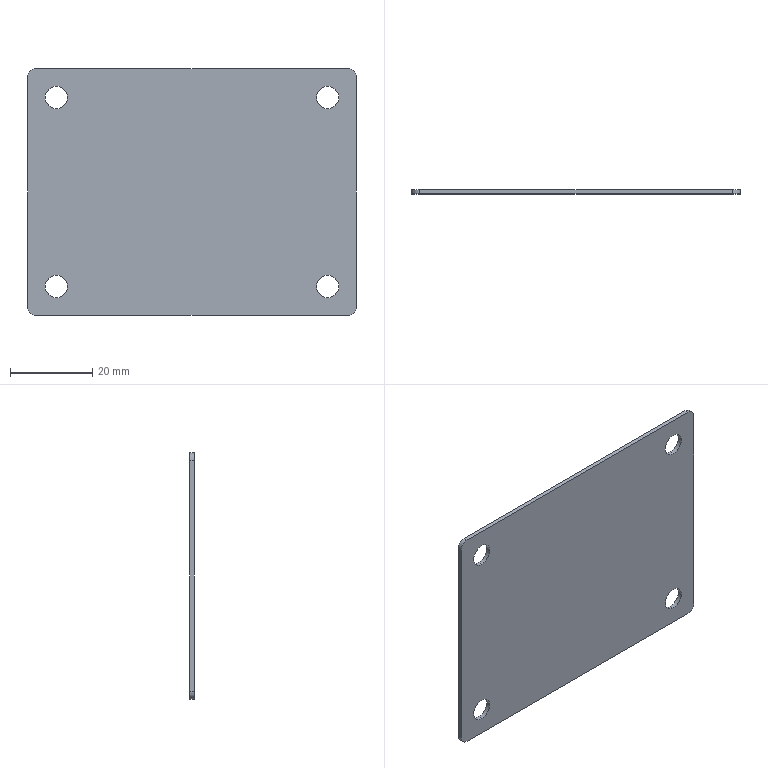Part | STEP file | 4060 profile end cover plate | 1 solid | 18 faces | box 80 x 1 x 60 mm | volume 4702 mm3 | cylinder 12 | plane 6 | commonest cylinder face diameters 5.5 x8 4 x4
STEP:
#1=CARTESIAN_POINT('',(0.,0.,0.));
#2=DIRECTION('',(0.,0.,1.));
#3=DIRECTION('',(1.,0.,0.));
#4=AXIS2_PLACEMENT_3D('',#1,#2,#3);
#5=CARTESIAN_POINT('',(33.,0.,-20.25));
#6=VERTEX_POINT('',#5);
#7=CARTESIAN_POINT('',(33.,1.,-20.25));
#8=VERTEX_POINT('',#7);
#9=CARTESIAN_POINT('',(33.,1.,-20.25));
#10=DIRECTION('',(0.,1.,0.));
#11=VECTOR('',#10,1.);
#12=LINE('',#9,#11);
#13=CARTESIAN_POINT('',(33.,1.,-23.));
#14=DIRECTION('',(0.,1.,0.));
#15=DIRECTION('',(0.,0.,1.));
#16=AXIS2_PLACEMENT_3D('',#13,#14,#15);
#17=CYLINDRICAL_SURFACE('',#16,2.75);
#18=CARTESIAN_POINT('',(6.283,0.));
#19=DIRECTION('',(0.,1.));
#20=VECTOR('',#19,1.);
#21=LINE('',#18,#20);
#22=(GEOMETRIC_REPRESENTATION_CONTEXT(2)PARAMETRIC_REPRESENTATION_CONTEXT()REPRESENTATION_CONTEXT('',''));
#23=DEFINITIONAL_REPRESENTATION('',(#21),#22);
#24=PCURVE('',#17,#23);
#25=CARTESIAN_POINT('',(33.,1.,-23.));
#26=DIRECTION('',(0.,1.,0.));
#27=DIRECTION('',(0.,0.,1.));
#28=AXIS2_PLACEMENT_3D('',#25,#26,#27);
#29=CYLINDRICAL_SURFACE('',#28,2.75);
#30=CARTESIAN_POINT('',(0.,0.));
#31=DIRECTION('',(0.,1.));
#32=VECTOR('',#31,1.);
#33=LINE('',#30,#32);
#34=(GEOMETRIC_REPRESENTATION_CONTEXT(2)PARAMETRIC_REPRESENTATION_CONTEXT()REPRESENTATION_CONTEXT('',''));
#35=DEFINITIONAL_REPRESENTATION('',(#33),#34);
#36=PCURVE('',#29,#35);
#37=SURFACE_CURVE('',#12,(#24,#36),.PCURVE_S1.);
#38=EDGE_CURVE('',#6,#8,#37,.T.);
#39=ORIENTED_EDGE('',*,*,#38,.T.);
#40=CARTESIAN_POINT('',(33.,1.,-25.75));
#41=VERTEX_POINT('',#40);
#42=CARTESIAN_POINT('',(33.,1.,-23.));
#43=DIRECTION('',(0.,1.,0.));
#44=DIRECTION('',(0.,0.,1.));
#45=AXIS2_PLACEMENT_3D('',#42,#43,#44);
#46=CIRCLE('',#45,2.75);
#47=CARTESIAN_POINT('',(0.,0.));
#48=DIRECTION('',(1.,0.));
#49=VECTOR('',#48,1.);
#50=LINE('',#47,#49);
#51=(GEOMETRIC_REPRESENTATION_CONTEXT(2)PARAMETRIC_REPRESENTATION_CONTEXT()REPRESENTATION_CONTEXT('',''));
#52=DEFINITIONAL_REPRESENTATION('',(#50),#51);
#53=PCURVE('',#17,#52);
#54=CARTESIAN_POINT('',(-38.,1.,28.));
#55=DIRECTION('',(0.,1.,0.));
#56=DIRECTION('',(0.,0.,1.));
#57=AXIS2_PLACEMENT_3D('',#54,#55,#56);
#58=PLANE('',#57);
#59=CARTESIAN_POINT('',(-51.,71.));
#60=DIRECTION('',(1.,0.));
#61=AXIS2_PLACEMENT_2D('',#59,#60);
#62=CIRCLE('',#61,2.75);
#63=(GEOMETRIC_REPRESENTATION_CONTEXT(2)PARAMETRIC_REPRESENTATION_CONTEXT()REPRESENTATION_CONTEXT('',''));
#64=DEFINITIONAL_REPRESENTATION('',(#62),#63);
#65=PCURVE('',#58,#64);
#66=SURFACE_CURVE('',#46,(#53,#65),.PCURVE_S1.);
#67=EDGE_CURVE('',#41,#8,#66,.T.);
#68=ORIENTED_EDGE('',*,*,#67,.F.);
#69=CARTESIAN_POINT('',(33.,0.,-25.75));
#70=VERTEX_POINT('',#69);
#71=CARTESIAN_POINT('',(33.,1.,-25.75));
#72=DIRECTION('',(0.,1.,0.));
#73=VECTOR('',#72,1.);
#74=LINE('',#71,#73);
#75=CARTESIAN_POINT('',(3.142,0.));
#76=DIRECTION('',(0.,1.));
#77=VECTOR('',#76,1.);
#78=LINE('',#75,#77);
#79=(GEOMETRIC_REPRESENTATION_CONTEXT(2)PARAMETRIC_REPRESENTATION_CONTEXT()REPRESENTATION_CONTEXT('',''));
#80=DEFINITIONAL_REPRESENTATION('',(#78),#79);
#81=PCURVE('',#17,#80);
#82=CARTESIAN_POINT('',(3.142,0.));
#83=DIRECTION('',(0.,1.));
#84=VECTOR('',#83,1.);
#85=LINE('',#82,#84);
#86=(GEOMETRIC_REPRESENTATION_CONTEXT(2)PARAMETRIC_REPRESENTATION_CONTEXT()REPRESENTATION_CONTEXT('',''));
#87=DEFINITIONAL_REPRESENTATION('',(#85),#86);
#88=PCURVE('',#29,#87);
#89=SURFACE_CURVE('',#74,(#81,#88),.PCURVE_S1.);
#90=EDGE_CURVE('',#70,#41,#89,.T.);
#91=ORIENTED_EDGE('',*,*,#90,.F.);
#92=CARTESIAN_POINT('',(33.,0.,-23.));
#93=DIRECTION('',(0.,1.,0.));
#94=DIRECTION('',(0.,0.,1.));
#95=AXIS2_PLACEMENT_3D('',#92,#93,#94);
#96=CIRCLE('',#95,2.75);
#97=CARTESIAN_POINT('',(0.,-1.));
#98=DIRECTION('',(1.,0.));
#99=VECTOR('',#98,1.);
#100=LINE('',#97,#99);
#101=(GEOMETRIC_REPRESENTATION_CONTEXT(2)PARAMETRIC_REPRESENTATION_CONTEXT()REPRESENTATION_CONTEXT('',''));
#102=DEFINITIONAL_REPRESENTATION('',(#100),#101);
#103=PCURVE('',#17,#102);
#104=CARTESIAN_POINT('',(-38.,0.,28.));
#105=DIRECTION('',(0.,1.,0.));
#106=DIRECTION('',(0.,0.,1.));
#107=AXIS2_PLACEMENT_3D('',#104,#105,#106);
#108=PLANE('',#107);
#109=CARTESIAN_POINT('',(-51.,71.));
#110=DIRECTION('',(1.,0.));
#111=AXIS2_PLACEMENT_2D('',#109,#110);
#112=CIRCLE('',#111,2.75);
#113=(GEOMETRIC_REPRESENTATION_CONTEXT(2)PARAMETRIC_REPRESENTATION_CONTEXT()REPRESENTATION_CONTEXT('',''));
#114=DEFINITIONAL_REPRESENTATION('',(#112),#113);
#115=PCURVE('',#108,#114);
#116=SURFACE_CURVE('',#96,(#103,#115),.PCURVE_S1.);
#117=EDGE_CURVE('',#70,#6,#116,.T.);
#118=ORIENTED_EDGE('',*,*,#117,.T.);
#119=EDGE_LOOP('',(#39,#68,#91,#118));
#120=FACE_BOUND('',#119,.F.);
#121=ADVANCED_FACE('',(#120),#17,.F.);
#122=CARTESIAN_POINT('',(-33.,0.,25.75));
#123=VERTEX_POINT('',#122);
#124=CARTESIAN_POINT('',(-33.,1.,25.75));
#125=VERTEX_POINT('',#124);
#126=CARTESIAN_POINT('',(-33.,1.,25.75));
#127=DIRECTION('',(0.,1.,0.));
#128=VECTOR('',#127,1.);
#129=LINE('',#126,#128);
#130=CARTESIAN_POINT('',(-33.,1.,23.));
#131=DIRECTION('',(0.,1.,0.));
#132=DIRECTION('',(0.,0.,1.));
#133=AXIS2_PLACEMENT_3D('',#130,#131,#132);
#134=CYLINDRICAL_SURFACE('',#133,2.75);
#135=CARTESIAN_POINT('',(6.283,0.));
#136=DIRECTION('',(0.,1.));
#137=VECTOR('',#136,1.);
#138=LINE('',#135,#137);
#139=(GEOMETRIC_REPRESENTATION_CONTEXT(2)PARAMETRIC_REPRESENTATION_CONTEXT()REPRESENTATION_CONTEXT('',''));
#140=DEFINITIONAL_REPRESENTATION('',(#138),#139);
#141=PCURVE('',#134,#140);
#142=CARTESIAN_POINT('',(-33.,1.,23.));
#143=DIRECTION('',(0.,1.,0.));
#144=DIRECTION('',(0.,0.,1.));
#145=AXIS2_PLACEMENT_3D('',#142,#143,#144);
#146=CYLINDRICAL_SURFACE('',#145,2.75);
#147=CARTESIAN_POINT('',(0.,0.));
#148=DIRECTION('',(0.,1.));
#149=VECTOR('',#148,1.);
#150=LINE('',#147,#149);
#151=(GEOMETRIC_REPRESENTATION_CONTEXT(2)PARAMETRIC_REPRESENTATION_CONTEXT()REPRESENTATION_CONTEXT('',''));
#152=DEFINITIONAL_REPRESENTATION('',(#150),#151);
#153=PCURVE('',#146,#152);
#154=SURFACE_CURVE('',#129,(#141,#153),.PCURVE_S1.);
#155=EDGE_CURVE('',#123,#125,#154,.T.);
#156=ORIENTED_EDGE('',*,*,#155,.T.);
#157=CARTESIAN_POINT('',(-33.,1.,20.25));
#158=VERTEX_POINT('',#157);
#159=CARTESIAN_POINT('',(-33.,1.,23.));
#160=DIRECTION('',(0.,1.,0.));
#161=DIRECTION('',(0.,0.,1.));
#162=AXIS2_PLACEMENT_3D('',#159,#160,#161);
#163=CIRCLE('',#162,2.75);
#164=CARTESIAN_POINT('',(0.,0.));
#165=DIRECTION('',(1.,0.));
#166=VECTOR('',#165,1.);
#167=LINE('',#164,#166);
#168=(GEOMETRIC_REPRESENTATION_CONTEXT(2)PARAMETRIC_REPRESENTATION_CONTEXT()REPRESENTATION_CONTEXT('',''));
#169=DEFINITIONAL_REPRESENTATION('',(#167),#168);
#170=PCURVE('',#134,#169);
#171=CARTESIAN_POINT('',(-5.,5.));
#172=DIRECTION('',(1.,0.));
#173=AXIS2_PLACEMENT_2D('',#171,#172);
#174=CIRCLE('',#173,2.75);
#175=(GEOMETRIC_REPRESENTATION_CONTEXT(2)PARAMETRIC_REPRESENTATION_CONTEXT()REPRESENTATION_CONTEXT('',''));
#176=DEFINITIONAL_REPRESENTATION('',(#174),#175);
#177=PCURVE('',#58,#176);
#178=SURFACE_CURVE('',#163,(#170,#177),.PCURVE_S1.);
#179=EDGE_CURVE('',#158,#125,#178,.T.);
#180=ORIENTED_EDGE('',*,*,#179,.F.);
#181=CARTESIAN_POINT('',(-33.,0.,20.25));
#182=VERTEX_POINT('',#181);
#183=CARTESIAN_POINT('',(-33.,1.,20.25));
#184=DIRECTION('',(0.,1.,0.));
#185=VECTOR('',#184,1.);
#186=LINE('',#183,#185);
#187=CARTESIAN_POINT('',(3.142,0.));
#188=DIRECTION('',(0.,1.));
#189=VECTOR('',#188,1.);
#190=LINE('',#187,#189);
#191=(GEOMETRIC_REPRESENTATION_CONTEXT(2)PARAMETRIC_REPRESENTATION_CONTEXT()REPRESENTATION_CONTEXT('',''));
#192=DEFINITIONAL_REPRESENTATION('',(#190),#191);
#193=PCURVE('',#134,#192);
#194=CARTESIAN_POINT('',(3.142,0.));
#195=DIRECTION('',(0.,1.));
#196=VECTOR('',#195,1.);
#197=LINE('',#194,#196);
#198=(GEOMETRIC_REPRESENTATION_CONTEXT(2)PARAMETRIC_REPRESENTATION_CONTEXT()REPRESENTATION_CONTEXT('',''));
#199=DEFINITIONAL_REPRESENTATION('',(#197),#198);
#200=PCURVE('',#146,#199);
#201=SURFACE_CURVE('',#186,(#193,#200),.PCURVE_S1.);
#202=EDGE_CURVE('',#182,#158,#201,.T.);
#203=ORIENTED_EDGE('',*,*,#202,.F.);
#204=CARTESIAN_POINT('',(-33.,0.,23.));
#205=DIRECTION('',(0.,1.,0.));
#206=DIRECTION('',(0.,0.,1.));
#207=AXIS2_PLACEMENT_3D('',#204,#205,#206);
#208=CIRCLE('',#207,2.75);
#209=CARTESIAN_POINT('',(0.,-1.));
#210=DIRECTION('',(1.,0.));
#211=VECTOR('',#210,1.);
#212=LINE('',#209,#211);
#213=(GEOMETRIC_REPRESENTATION_CONTEXT(2)PARAMETRIC_REPRESENTATION_CONTEXT()REPRESENTATION_CONTEXT('',''));
#214=DEFINITIONAL_REPRESENTATION('',(#212),#213);
#215=PCURVE('',#134,#214);
#216=CARTESIAN_POINT('',(-5.,5.));
#217=DIRECTION('',(1.,0.));
#218=AXIS2_PLACEMENT_2D('',#216,#217);
#219=CIRCLE('',#218,2.75);
#220=(GEOMETRIC_REPRESENTATION_CONTEXT(2)PARAMETRIC_REPRESENTATION_CONTEXT()REPRESENTATION_CONTEXT('',''));
#221=DEFINITIONAL_REPRESENTATION('',(#219),#220);
#222=PCURVE('',#108,#221);
#223=SURFACE_CURVE('',#208,(#215,#222),.PCURVE_S1.);
#224=EDGE_CURVE('',#182,#123,#223,.T.);
#225=ORIENTED_EDGE('',*,*,#224,.T.);
#226=EDGE_LOOP('',(#156,#180,#203,#225));
#227=FACE_BOUND('',#226,.F.);
#228=ADVANCED_FACE('',(#227),#134,.F.);
#229=CARTESIAN_POINT('',(-33.,0.,-20.25));
#230=VERTEX_POINT('',#229);
#231=CARTESIAN_POINT('',(-33.,1.,-20.25));
#232=VERTEX_POINT('',#231);
#233=CARTESIAN_POINT('',(-33.,1.,-20.25));
#234=DIRECTION('',(0.,1.,0.));
#235=VECTOR('',#234,1.);
#236=LINE('',#233,#235);
#237=CARTESIAN_POINT('',(-33.,1.,-23.));
#238=DIRECTION('',(0.,1.,0.));
#239=DIRECTION('',(0.,0.,1.));
#240=AXIS2_PLACEMENT_3D('',#237,#238,#239);
#241=CYLINDRICAL_SURFACE('',#240,2.75);
#242=CARTESIAN_POINT('',(6.283,0.));
#243=DIRECTION('',(0.,1.));
#244=VECTOR('',#243,1.);
#245=LINE('',#242,#244);
#246=(GEOMETRIC_REPRESENTATION_CONTEXT(2)PARAMETRIC_REPRESENTATION_CONTEXT()REPRESENTATION_CONTEXT('',''));
#247=DEFINITIONAL_REPRESENTATION('',(#245),#246);
#248=PCURVE('',#241,#247);
#249=CARTESIAN_POINT('',(-33.,1.,-23.));
#250=DIRECTION('',(0.,1.,0.));
#251=DIRECTION('',(0.,0.,1.));
#252=AXIS2_PLACEMENT_3D('',#249,#250,#251);
#253=CYLINDRICAL_SURFACE('',#252,2.75);
#254=CARTESIAN_POINT('',(0.,0.));
#255=DIRECTION('',(0.,1.));
#256=VECTOR('',#255,1.);
#257=LINE('',#254,#256);
#258=(GEOMETRIC_REPRESENTATION_CONTEXT(2)PARAMETRIC_REPRESENTATION_CONTEXT()REPRESENTATION_CONTEXT('',''));
#259=DEFINITIONAL_REPRESENTATION('',(#257),#258);
#260=PCURVE('',#253,#259);
#261=SURFACE_CURVE('',#236,(#248,#260),.PCURVE_S1.);
#262=EDGE_CURVE('',#230,#232,#261,.T.);
#263=ORIENTED_EDGE('',*,*,#262,.T.);
#264=CARTESIAN_POINT('',(-33.,1.,-25.75));
#265=VERTEX_POINT('',#264);
#266=CARTESIAN_POINT('',(-33.,1.,-23.));
#267=DIRECTION('',(0.,1.,0.));
#268=DIRECTION('',(0.,0.,1.));
#269=AXIS2_PLACEMENT_3D('',#266,#267,#268);
#270=CIRCLE('',#269,2.75);
#271=CARTESIAN_POINT('',(0.,0.));
#272=DIRECTION('',(1.,0.));
#273=VECTOR('',#272,1.);
#274=LINE('',#271,#273);
#275=(GEOMETRIC_REPRESENTATION_CONTEXT(2)PARAMETRIC_REPRESENTATION_CONTEXT()REPRESENTATION_CONTEXT('',''));
#276=DEFINITIONAL_REPRESENTATION('',(#274),#275);
#277=PCURVE('',#241,#276);
#278=CARTESIAN_POINT('',(-51.,5.));
#279=DIRECTION('',(1.,0.));
#280=AXIS2_PLACEMENT_2D('',#278,#279);
#281=CIRCLE('',#280,2.75);
#282=(GEOMETRIC_REPRESENTATION_CONTEXT(2)PARAMETRIC_REPRESENTATION_CONTEXT()REPRESENTATION_CONTEXT('',''));
#283=DEFINITIONAL_REPRESENTATION('',(#281),#282);
#284=PCURVE('',#58,#283);
#285=SURFACE_CURVE('',#270,(#277,#284),.PCURVE_S1.);
#286=EDGE_CURVE('',#265,#232,#285,.T.);
#287=ORIENTED_EDGE('',*,*,#286,.F.);
#288=CARTESIAN_POINT('',(-33.,0.,-25.75));
#289=VERTEX_POINT('',#288);
#290=CARTESIAN_POINT('',(-33.,1.,-25.75));
#291=DIRECTION('',(0.,1.,0.));
#292=VECTOR('',#291,1.);
#293=LINE('',#290,#292);
#294=CARTESIAN_POINT('',(3.142,0.));
#295=DIRECTION('',(0.,1.));
#296=VECTOR('',#295,1.);
#297=LINE('',#294,#296);
#298=(GEOMETRIC_REPRESENTATION_CONTEXT(2)PARAMETRIC_REPRESENTATION_CONTEXT()REPRESENTATION_CONTEXT('',''));
#299=DEFINITIONAL_REPRESENTATION('',(#297),#298);
#300=PCURVE('',#241,#299);
#301=CARTESIAN_POINT('',(3.142,0.));
#302=DIRECTION('',(0.,1.));
#303=VECTOR('',#302,1.);
#304=LINE('',#301,#303);
#305=(GEOMETRIC_REPRESENTATION_CONTEXT(2)PARAMETRIC_REPRESENTATION_CONTEXT()REPRESENTATION_CONTEXT('',''));
#306=DEFINITIONAL_REPRESENTATION('',(#304),#305);
#307=PCURVE('',#253,#306);
#308=SURFACE_CURVE('',#293,(#300,#307),.PCURVE_S1.);
#309=EDGE_CURVE('',#289,#265,#308,.T.);
#310=ORIENTED_EDGE('',*,*,#309,.F.);
#311=CARTESIAN_POINT('',(-33.,0.,-23.));
#312=DIRECTION('',(0.,1.,0.));
#313=DIRECTION('',(0.,0.,1.));
#314=AXIS2_PLACEMENT_3D('',#311,#312,#313);
#315=CIRCLE('',#314,2.75);
#316=CARTESIAN_POINT('',(0.,-1.));
#317=DIRECTION('',(1.,0.));
#318=VECTOR('',#317,1.);
#319=LINE('',#316,#318);
#320=(GEOMETRIC_REPRESENTATION_CONTEXT(2)PARAMETRIC_REPRESENTATION_CONTEXT()REPRESENTATION_CONTEXT('',''));
#321=DEFINITIONAL_REPRESENTATION('',(#319),#320);
#322=PCURVE('',#241,#321);
#323=CARTESIAN_POINT('',(-51.,5.));
#324=DIRECTION('',(1.,0.));
#325=AXIS2_PLACEMENT_2D('',#323,#324);
#326=CIRCLE('',#325,2.75);
#327=(GEOMETRIC_REPRESENTATION_CONTEXT(2)PARAMETRIC_REPRESENTATION_CONTEXT()REPRESENTATION_CONTEXT('',''));
#328=DEFINITIONAL_REPRESENTATION('',(#326),#327);
#329=PCURVE('',#108,#328);
#330=SURFACE_CURVE('',#315,(#322,#329),.PCURVE_S1.);
#331=EDGE_CURVE('',#289,#230,#330,.T.);
#332=ORIENTED_EDGE('',*,*,#331,.T.);
#333=EDGE_LOOP('',(#263,#287,#310,#332));
#334=FACE_BOUND('',#333,.F.);
#335=ADVANCED_FACE('',(#334),#241,.F.);
#336=CARTESIAN_POINT('',(33.,0.,25.75));
#337=VERTEX_POINT('',#336);
#338=CARTESIAN_POINT('',(33.,1.,25.75));
#339=VERTEX_POINT('',#338);
#340=CARTESIAN_POINT('',(33.,1.,25.75));
#341=DIRECTION('',(0.,1.,0.));
#342=VECTOR('',#341,1.);
#343=LINE('',#340,#342);
#344=CARTESIAN_POINT('',(33.,1.,23.));
#345=DIRECTION('',(0.,1.,0.));
#346=DIRECTION('',(0.,0.,1.));
#347=AXIS2_PLACEMENT_3D('',#344,#345,#346);
#348=CYLINDRICAL_SURFACE('',#347,2.75);
#349=CARTESIAN_POINT('',(6.283,0.));
#350=DIRECTION('',(0.,1.));
#351=VECTOR('',#350,1.);
#352=LINE('',#349,#351);
#353=(GEOMETRIC_REPRESENTATION_CONTEXT(2)PARAMETRIC_REPRESENTATION_CONTEXT()REPRESENTATION_CONTEXT('',''));
#354=DEFINITIONAL_REPRESENTATION('',(#352),#353);
#355=PCURVE('',#348,#354);
#356=CARTESIAN_POINT('',(33.,1.,23.));
#357=DIRECTION('',(0.,1.,0.));
#358=DIRECTION('',(0.,0.,1.));
#359=AXIS2_PLACEMENT_3D('',#356,#357,#358);
#360=CYLINDRICAL_SURFACE('',#359,2.75);
#361=CARTESIAN_POINT('',(0.,0.));
#362=DIRECTION('',(0.,1.));
#363=VECTOR('',#362,1.);
#364=LINE('',#361,#363);
#365=(GEOMETRIC_REPRESENTATION_CONTEXT(2)PARAMETRIC_REPRESENTATION_CONTEXT()REPRESENTATION_CONTEXT('',''));
#366=DEFINITIONAL_REPRESENTATION('',(#364),#365);
#367=PCURVE('',#360,#366);
#368=SURFACE_CURVE('',#343,(#355,#367),.PCURVE_S1.);
#369=EDGE_CURVE('',#337,#339,#368,.T.);
#370=ORIENTED_EDGE('',*,*,#369,.T.);
#371=CARTESIAN_POINT('',(33.,1.,20.25));
#372=VERTEX_POINT('',#371);
#373=CARTESIAN_POINT('',(33.,1.,23.));
#374=DIRECTION('',(0.,1.,0.));
#375=DIRECTION('',(0.,0.,1.));
#376=AXIS2_PLACEMENT_3D('',#373,#374,#375);
#377=CIRCLE('',#376,2.75);
#378=CARTESIAN_POINT('',(0.,0.));
#379=DIRECTION('',(1.,0.));
#380=VECTOR('',#379,1.);
#381=LINE('',#378,#380);
#382=(GEOMETRIC_REPRESENTATION_CONTEXT(2)PARAMETRIC_REPRESENTATION_CONTEXT()REPRESENTATION_CONTEXT('',''));
#383=DEFINITIONAL_REPRESENTATION('',(#381),#382);
#384=PCURVE('',#348,#383);
#385=CARTESIAN_POINT('',(-5.,71.));
#386=DIRECTION('',(1.,0.));
#387=AXIS2_PLACEMENT_2D('',#385,#386);
#388=CIRCLE('',#387,2.75);
#389=(GEOMETRIC_REPRESENTATION_CONTEXT(2)PARAMETRIC_REPRESENTATION_CONTEXT()REPRESENTATION_CONTEXT('',''));
#390=DEFINITIONAL_REPRESENTATION('',(#388),#389);
#391=PCURVE('',#58,#390);
#392=SURFACE_CURVE('',#377,(#384,#391),.PCURVE_S1.);
#393=EDGE_CURVE('',#372,#339,#392,.T.);
#394=ORIENTED_EDGE('',*,*,#393,.F.);
#395=CARTESIAN_POINT('',(33.,0.,20.25));
#396=VERTEX_POINT('',#395);
#397=CARTESIAN_POINT('',(33.,1.,20.25));
#398=DIRECTION('',(0.,1.,0.));
#399=VECTOR('',#398,1.);
#400=LINE('',#397,#399);
#401=CARTESIAN_POINT('',(3.142,0.));
#402=DIRECTION('',(0.,1.));
#403=VECTOR('',#402,1.);
#404=LINE('',#401,#403);
#405=(GEOMETRIC_REPRESENTATION_CONTEXT(2)PARAMETRIC_REPRESENTATION_CONTEXT()REPRESENTATION_CONTEXT('',''));
#406=DEFINITIONAL_REPRESENTATION('',(#404),#405);
#407=PCURVE('',#348,#406);
#408=CARTESIAN_POINT('',(3.142,0.));
#409=DIRECTION('',(0.,1.));
#410=VECTOR('',#409,1.);
#411=LINE('',#408,#410);
#412=(GEOMETRIC_REPRESENTATION_CONTEXT(2)PARAMETRIC_REPRESENTATION_CONTEXT()REPRESENTATION_CONTEXT('',''));
#413=DEFINITIONAL_REPRESENTATION('',(#411),#412);
#414=PCURVE('',#360,#413);
#415=SURFACE_CURVE('',#400,(#407,#414),.PCURVE_S1.);
#416=EDGE_CURVE('',#396,#372,#415,.T.);
#417=ORIENTED_EDGE('',*,*,#416,.F.);
#418=CARTESIAN_POINT('',(33.,0.,23.));
#419=DIRECTION('',(0.,1.,0.));
#420=DIRECTION('',(0.,0.,1.));
#421=AXIS2_PLACEMENT_3D('',#418,#419,#420);
#422=CIRCLE('',#421,2.75);
#423=CARTESIAN_POINT('',(0.,-1.));
#424=DIRECTION('',(1.,0.));
#425=VECTOR('',#424,1.);
#426=LINE('',#423,#425);
#427=(GEOMETRIC_REPRESENTATION_CONTEXT(2)PARAMETRIC_REPRESENTATION_CONTEXT()REPRESENTATION_CONTEXT('',''));
#428=DEFINITIONAL_REPRESENTATION('',(#426),#427);
#429=PCURVE('',#348,#428);
#430=CARTESIAN_POINT('',(-5.,71.));
#431=DIRECTION('',(1.,0.));
#432=AXIS2_PLACEMENT_2D('',#430,#431);
#433=CIRCLE('',#432,2.75);
#434=(GEOMETRIC_REPRESENTATION_CONTEXT(2)PARAMETRIC_REPRESENTATION_CONTEXT()REPRESENTATION_CONTEXT('',''));
#435=DEFINITIONAL_REPRESENTATION('',(#433),#434);
#436=PCURVE('',#108,#435);
#437=SURFACE_CURVE('',#422,(#429,#436),.PCURVE_S1.);
#438=EDGE_CURVE('',#396,#337,#437,.T.);
#439=ORIENTED_EDGE('',*,*,#438,.T.);
#440=EDGE_LOOP('',(#370,#394,#417,#439));
#441=FACE_BOUND('',#440,.F.);
#442=ADVANCED_FACE('',(#441),#348,.F.);
#443=CARTESIAN_POINT('',(-40.,0.,28.));
#444=VERTEX_POINT('',#443);
#445=CARTESIAN_POINT('',(-38.,0.,30.));
#446=VERTEX_POINT('',#445);
#447=CARTESIAN_POINT('',(-38.,0.,28.));
#448=DIRECTION('',(0.,1.,0.));
#449=DIRECTION('',(0.,0.,1.));
#450=AXIS2_PLACEMENT_3D('',#447,#448,#449);
#451=CIRCLE('',#450,2.);
#452=CARTESIAN_POINT('',(-38.,1.,28.));
#453=DIRECTION('',(0.,-1.,0.));
#454=DIRECTION('',(0.,0.,-1.));
#455=AXIS2_PLACEMENT_3D('',#452,#453,#454);
#456=CYLINDRICAL_SURFACE('',#455,2.);
#457=CARTESIAN_POINT('',(9.425,1.));
#458=DIRECTION('',(-1.,0.));
#459=VECTOR('',#458,1.);
#460=LINE('',#457,#459);
#461=(GEOMETRIC_REPRESENTATION_CONTEXT(2)PARAMETRIC_REPRESENTATION_CONTEXT()REPRESENTATION_CONTEXT('',''));
#462=DEFINITIONAL_REPRESENTATION('',(#460),#461);
#463=PCURVE('',#456,#462);
#464=CARTESIAN_POINT('',(0.,0.));
#465=DIRECTION('',(1.,0.));
#466=AXIS2_PLACEMENT_2D('',#464,#465);
#467=CIRCLE('',#466,2.);
#468=(GEOMETRIC_REPRESENTATION_CONTEXT(2)PARAMETRIC_REPRESENTATION_CONTEXT()REPRESENTATION_CONTEXT('',''));
#469=DEFINITIONAL_REPRESENTATION('',(#467),#468);
#470=PCURVE('',#108,#469);
#471=SURFACE_CURVE('',#451,(#463,#470),.PCURVE_S1.);
#472=EDGE_CURVE('',#444,#446,#471,.T.);
#473=ORIENTED_EDGE('',*,*,#472,.T.);
#474=CARTESIAN_POINT('',(-38.,1.,30.));
#475=VERTEX_POINT('',#474);
#476=CARTESIAN_POINT('',(-38.,1.,30.));
#477=DIRECTION('',(0.,-1.,0.));
#478=VECTOR('',#477,1.);
#479=LINE('',#476,#478);
#480=CARTESIAN_POINT('',(3.142,0.));
#481=DIRECTION('',(0.,1.));
#482=VECTOR('',#481,1.);
#483=LINE('',#480,#482);
#484=(GEOMETRIC_REPRESENTATION_CONTEXT(2)PARAMETRIC_REPRESENTATION_CONTEXT()REPRESENTATION_CONTEXT('',''));
#485=DEFINITIONAL_REPRESENTATION('',(#483),#484);
#486=PCURVE('',#456,#485);
#487=CARTESIAN_POINT('',(-38.,1.,30.));
#488=DIRECTION('',(0.,0.,-1.));
#489=DIRECTION('',(-1.,0.,0.));
#490=AXIS2_PLACEMENT_3D('',#487,#488,#489);
#491=PLANE('',#490);
#492=CARTESIAN_POINT('',(0.,0.));
#493=DIRECTION('',(0.,-1.));
#494=VECTOR('',#493,1.);
#495=LINE('',#492,#494);
#496=(GEOMETRIC_REPRESENTATION_CONTEXT(2)PARAMETRIC_REPRESENTATION_CONTEXT()REPRESENTATION_CONTEXT('',''));
#497=DEFINITIONAL_REPRESENTATION('',(#495),#496);
#498=PCURVE('',#491,#497);
#499=SURFACE_CURVE('',#479,(#486,#498),.PCURVE_S1.);
#500=EDGE_CURVE('',#475,#446,#499,.T.);
#501=ORIENTED_EDGE('',*,*,#500,.F.);
#502=CARTESIAN_POINT('',(-40.,1.,28.));
#503=VERTEX_POINT('',#502);
#504=CARTESIAN_POINT('',(-38.,1.,28.));
#505=DIRECTION('',(0.,1.,0.));
#506=DIRECTION('',(0.,0.,1.));
#507=AXIS2_PLACEMENT_3D('',#504,#505,#506);
#508=CIRCLE('',#507,2.);
#509=CARTESIAN_POINT('',(9.425,0.));
#510=DIRECTION('',(-1.,0.));
#511=VECTOR('',#510,1.);
#512=LINE('',#509,#511);
#513=(GEOMETRIC_REPRESENTATION_CONTEXT(2)PARAMETRIC_REPRESENTATION_CONTEXT()REPRESENTATION_CONTEXT('',''));
#514=DEFINITIONAL_REPRESENTATION('',(#512),#513);
#515=PCURVE('',#456,#514);
#516=CARTESIAN_POINT('',(0.,0.));
#517=DIRECTION('',(1.,0.));
#518=AXIS2_PLACEMENT_2D('',#516,#517);
#519=CIRCLE('',#518,2.);
#520=(GEOMETRIC_REPRESENTATION_CONTEXT(2)PARAMETRIC_REPRESENTATION_CONTEXT()REPRESENTATION_CONTEXT('',''));
#521=DEFINITIONAL_REPRESENTATION('',(#519),#520);
#522=PCURVE('',#58,#521);
#523=SURFACE_CURVE('',#508,(#515,#522),.PCURVE_S1.);
#524=EDGE_CURVE('',#503,#475,#523,.T.);
#525=ORIENTED_EDGE('',*,*,#524,.F.);
#526=CARTESIAN_POINT('',(-40.,1.,28.));
#527=DIRECTION('',(0.,-1.,0.));
#528=VECTOR('',#527,1.);
#529=LINE('',#526,#528);
#530=CARTESIAN_POINT('',(4.712,0.));
#531=DIRECTION('',(0.,1.));
#532=VECTOR('',#531,1.);
#533=LINE('',#530,#532);
#534=(GEOMETRIC_REPRESENTATION_CONTEXT(2)PARAMETRIC_REPRESENTATION_CONTEXT()REPRESENTATION_CONTEXT('',''));
#535=DEFINITIONAL_REPRESENTATION('',(#533),#534);
#536=PCURVE('',#456,#535);
#537=CARTESIAN_POINT('',(-40.,1.,-28.));
#538=DIRECTION('',(1.,0.,0.));
#539=DIRECTION('',(0.,0.,-1.));
#540=AXIS2_PLACEMENT_3D('',#537,#538,#539);
#541=PLANE('',#540);
#542=CARTESIAN_POINT('',(-56.,0.));
#543=DIRECTION('',(0.,-1.));
#544=VECTOR('',#543,1.);
#545=LINE('',#542,#544);
#546=(GEOMETRIC_REPRESENTATION_CONTEXT(2)PARAMETRIC_REPRESENTATION_CONTEXT()REPRESENTATION_CONTEXT('',''));
#547=DEFINITIONAL_REPRESENTATION('',(#545),#546);
#548=PCURVE('',#541,#547);
#549=SURFACE_CURVE('',#529,(#536,#548),.PCURVE_S1.);
#550=EDGE_CURVE('',#503,#444,#549,.T.);
#551=ORIENTED_EDGE('',*,*,#550,.T.);
#552=EDGE_LOOP('',(#473,#501,#525,#551));
#553=FACE_BOUND('',#552,.T.);
#554=ADVANCED_FACE('',(#553),#456,.T.);
#555=CARTESIAN_POINT('',(38.,0.,30.));
#556=VERTEX_POINT('',#555);
#557=CARTESIAN_POINT('',(-38.,0.,30.));
#558=DIRECTION('',(1.,0.,0.));
#559=VECTOR('',#558,1.);
#560=LINE('',#557,#559);
#561=CARTESIAN_POINT('',(0.,-1.));
#562=DIRECTION('',(-1.,0.));
#563=VECTOR('',#562,1.);
#564=LINE('',#561,#563);
#565=(GEOMETRIC_REPRESENTATION_CONTEXT(2)PARAMETRIC_REPRESENTATION_CONTEXT()REPRESENTATION_CONTEXT('',''));
#566=DEFINITIONAL_REPRESENTATION('',(#564),#565);
#567=PCURVE('',#491,#566);
#568=CARTESIAN_POINT('',(2.,0.));
#569=DIRECTION('',(0.,1.));
#570=VECTOR('',#569,1.);
#571=LINE('',#568,#570);
#572=(GEOMETRIC_REPRESENTATION_CONTEXT(2)PARAMETRIC_REPRESENTATION_CONTEXT()REPRESENTATION_CONTEXT('',''));
#573=DEFINITIONAL_REPRESENTATION('',(#571),#572);
#574=PCURVE('',#108,#573);
#575=SURFACE_CURVE('',#560,(#567,#574),.PCURVE_S1.);
#576=EDGE_CURVE('',#446,#556,#575,.T.);
#577=ORIENTED_EDGE('',*,*,#576,.T.);
#578=CARTESIAN_POINT('',(38.,1.,30.));
#579=VERTEX_POINT('',#578);
#580=CARTESIAN_POINT('',(38.,1.,30.));
#581=DIRECTION('',(0.,-1.,0.));
#582=VECTOR('',#581,1.);
#583=LINE('',#580,#582);
#584=CARTESIAN_POINT('',(-76.,0.));
#585=DIRECTION('',(0.,-1.));
#586=VECTOR('',#585,1.);
#587=LINE('',#584,#586);
#588=(GEOMETRIC_REPRESENTATION_CONTEXT(2)PARAMETRIC_REPRESENTATION_CONTEXT()REPRESENTATION_CONTEXT('',''));
#589=DEFINITIONAL_REPRESENTATION('',(#587),#588);
#590=PCURVE('',#491,#589);
#591=CARTESIAN_POINT('',(38.,1.,28.));
#592=DIRECTION('',(0.,-1.,0.));
#593=DIRECTION('',(0.,0.,-1.));
#594=AXIS2_PLACEMENT_3D('',#591,#592,#593);
#595=CYLINDRICAL_SURFACE('',#594,2.);
#596=CARTESIAN_POINT('',(3.142,0.));
#597=DIRECTION('',(0.,1.));
#598=VECTOR('',#597,1.);
#599=LINE('',#596,#598);
#600=(GEOMETRIC_REPRESENTATION_CONTEXT(2)PARAMETRIC_REPRESENTATION_CONTEXT()REPRESENTATION_CONTEXT('',''));
#601=DEFINITIONAL_REPRESENTATION('',(#599),#600);
#602=PCURVE('',#595,#601);
#603=SURFACE_CURVE('',#583,(#590,#602),.PCURVE_S1.);
#604=EDGE_CURVE('',#579,#556,#603,.T.);
#605=ORIENTED_EDGE('',*,*,#604,.F.);
#606=CARTESIAN_POINT('',(-38.,1.,30.));
#607=DIRECTION('',(1.,0.,0.));
#608=VECTOR('',#607,1.);
#609=LINE('',#606,#608);
#610=CARTESIAN_POINT('',(0.,0.));
#611=DIRECTION('',(-1.,0.));
#612=VECTOR('',#611,1.);
#613=LINE('',#610,#612);
#614=(GEOMETRIC_REPRESENTATION_CONTEXT(2)PARAMETRIC_REPRESENTATION_CONTEXT()REPRESENTATION_CONTEXT('',''));
#615=DEFINITIONAL_REPRESENTATION('',(#613),#614);
#616=PCURVE('',#491,#615);
#617=CARTESIAN_POINT('',(2.,0.));
#618=DIRECTION('',(0.,1.));
#619=VECTOR('',#618,1.);
#620=LINE('',#617,#619);
#621=(GEOMETRIC_REPRESENTATION_CONTEXT(2)PARAMETRIC_REPRESENTATION_CONTEXT()REPRESENTATION_CONTEXT('',''));
#622=DEFINITIONAL_REPRESENTATION('',(#620),#621);
#623=PCURVE('',#58,#622);
#624=SURFACE_CURVE('',#609,(#616,#623),.PCURVE_S1.);
#625=EDGE_CURVE('',#475,#579,#624,.T.);
#626=ORIENTED_EDGE('',*,*,#625,.F.);
#627=ORIENTED_EDGE('',*,*,#500,.T.);
#628=EDGE_LOOP('',(#577,#605,#626,#627));
#629=FACE_BOUND('',#628,.T.);
#630=ADVANCED_FACE('',(#629),#491,.F.);
#631=CARTESIAN_POINT('',(40.,0.,28.));
#632=VERTEX_POINT('',#631);
#633=CARTESIAN_POINT('',(38.,0.,28.));
#634=DIRECTION('',(0.,1.,0.));
#635=DIRECTION('',(0.,0.,1.));
#636=AXIS2_PLACEMENT_3D('',#633,#634,#635);
#637=CIRCLE('',#636,2.);
#638=CARTESIAN_POINT('',(3.142,1.));
#639=DIRECTION('',(-1.,0.));
#640=VECTOR('',#639,1.);
#641=LINE('',#638,#640);
#642=(GEOMETRIC_REPRESENTATION_CONTEXT(2)PARAMETRIC_REPRESENTATION_CONTEXT()REPRESENTATION_CONTEXT('',''));
#643=DEFINITIONAL_REPRESENTATION('',(#641),#642);
#644=PCURVE('',#595,#643);
#645=CARTESIAN_POINT('',(0.,76.));
#646=DIRECTION('',(1.,0.));
#647=AXIS2_PLACEMENT_2D('',#645,#646);
#648=CIRCLE('',#647,2.);
#649=(GEOMETRIC_REPRESENTATION_CONTEXT(2)PARAMETRIC_REPRESENTATION_CONTEXT()REPRESENTATION_CONTEXT('',''));
#650=DEFINITIONAL_REPRESENTATION('',(#648),#649);
#651=PCURVE('',#108,#650);
#652=SURFACE_CURVE('',#637,(#644,#651),.PCURVE_S1.);
#653=EDGE_CURVE('',#556,#632,#652,.T.);
#654=ORIENTED_EDGE('',*,*,#653,.T.);
#655=CARTESIAN_POINT('',(40.,1.,28.));
#656=VERTEX_POINT('',#655);
#657=CARTESIAN_POINT('',(40.,1.,28.));
#658=DIRECTION('',(0.,-1.,0.));
#659=VECTOR('',#658,1.);
#660=LINE('',#657,#659);
#661=CARTESIAN_POINT('',(1.571,0.));
#662=DIRECTION('',(0.,1.));
#663=VECTOR('',#662,1.);
#664=LINE('',#661,#663);
#665=(GEOMETRIC_REPRESENTATION_CONTEXT(2)PARAMETRIC_REPRESENTATION_CONTEXT()REPRESENTATION_CONTEXT('',''));
#666=DEFINITIONAL_REPRESENTATION('',(#664),#665);
#667=PCURVE('',#595,#666);
#668=CARTESIAN_POINT('',(40.,1.,-28.));
#669=DIRECTION('',(-1.,0.,0.));
#670=DIRECTION('',(0.,0.,1.));
#671=AXIS2_PLACEMENT_3D('',#668,#669,#670);
#672=PLANE('',#671);
#673=CARTESIAN_POINT('',(56.,0.));
#674=DIRECTION('',(0.,-1.));
#675=VECTOR('',#674,1.);
#676=LINE('',#673,#675);
#677=(GEOMETRIC_REPRESENTATION_CONTEXT(2)PARAMETRIC_REPRESENTATION_CONTEXT()REPRESENTATION_CONTEXT('',''));
#678=DEFINITIONAL_REPRESENTATION('',(#676),#677);
#679=PCURVE('',#672,#678);
#680=SURFACE_CURVE('',#660,(#667,#679),.PCURVE_S1.);
#681=EDGE_CURVE('',#656,#632,#680,.T.);
#682=ORIENTED_EDGE('',*,*,#681,.F.);
#683=CARTESIAN_POINT('',(38.,1.,28.));
#684=DIRECTION('',(0.,1.,0.));
#685=DIRECTION('',(0.,0.,1.));
#686=AXIS2_PLACEMENT_3D('',#683,#684,#685);
#687=CIRCLE('',#686,2.);
#688=CARTESIAN_POINT('',(3.142,0.));
#689=DIRECTION('',(-1.,0.));
#690=VECTOR('',#689,1.);
#691=LINE('',#688,#690);
#692=(GEOMETRIC_REPRESENTATION_CONTEXT(2)PARAMETRIC_REPRESENTATION_CONTEXT()REPRESENTATION_CONTEXT('',''));
#693=DEFINITIONAL_REPRESENTATION('',(#691),#692);
#694=PCURVE('',#595,#693);
#695=CARTESIAN_POINT('',(0.,76.));
#696=DIRECTION('',(1.,0.));
#697=AXIS2_PLACEMENT_2D('',#695,#696);
#698=CIRCLE('',#697,2.);
#699=(GEOMETRIC_REPRESENTATION_CONTEXT(2)PARAMETRIC_REPRESENTATION_CONTEXT()REPRESENTATION_CONTEXT('',''));
#700=DEFINITIONAL_REPRESENTATION('',(#698),#699);
#701=PCURVE('',#58,#700);
#702=SURFACE_CURVE('',#687,(#694,#701),.PCURVE_S1.);
#703=EDGE_CURVE('',#579,#656,#702,.T.);
#704=ORIENTED_EDGE('',*,*,#703,.F.);
#705=ORIENTED_EDGE('',*,*,#604,.T.);
#706=EDGE_LOOP('',(#654,#682,#704,#705));
#707=FACE_BOUND('',#706,.T.);
#708=ADVANCED_FACE('',(#707),#595,.T.);
#709=CARTESIAN_POINT('',(40.,0.,-28.));
#710=VERTEX_POINT('',#709);
#711=CARTESIAN_POINT('',(40.,0.,-28.));
#712=DIRECTION('',(0.,0.,-1.));
#713=VECTOR('',#712,1.);
#714=LINE('',#711,#713);
#715=CARTESIAN_POINT('',(0.,-1.));
#716=DIRECTION('',(-1.,0.));
#717=VECTOR('',#716,1.);
#718=LINE('',#715,#717);
#719=(GEOMETRIC_REPRESENTATION_CONTEXT(2)PARAMETRIC_REPRESENTATION_CONTEXT()REPRESENTATION_CONTEXT('',''));
#720=DEFINITIONAL_REPRESENTATION('',(#718),#719);
#721=PCURVE('',#672,#720);
#722=CARTESIAN_POINT('',(-56.,78.));
#723=DIRECTION('',(-1.,0.));
#724=VECTOR('',#723,1.);
#725=LINE('',#722,#724);
#726=(GEOMETRIC_REPRESENTATION_CONTEXT(2)PARAMETRIC_REPRESENTATION_CONTEXT()REPRESENTATION_CONTEXT('',''));
#727=DEFINITIONAL_REPRESENTATION('',(#725),#726);
#728=PCURVE('',#108,#727);
#729=SURFACE_CURVE('',#714,(#721,#728),.PCURVE_S1.);
#730=EDGE_CURVE('',#632,#710,#729,.T.);
#731=ORIENTED_EDGE('',*,*,#730,.T.);
#732=CARTESIAN_POINT('',(40.,1.,-28.));
#733=VERTEX_POINT('',#732);
#734=CARTESIAN_POINT('',(40.,1.,-28.));
#735=DIRECTION('',(0.,-1.,0.));
#736=VECTOR('',#735,1.);
#737=LINE('',#734,#736);
#738=CARTESIAN_POINT('',(0.,0.));
#739=DIRECTION('',(0.,-1.));
#740=VECTOR('',#739,1.);
#741=LINE('',#738,#740);
#742=(GEOMETRIC_REPRESENTATION_CONTEXT(2)PARAMETRIC_REPRESENTATION_CONTEXT()REPRESENTATION_CONTEXT('',''));
#743=DEFINITIONAL_REPRESENTATION('',(#741),#742);
#744=PCURVE('',#672,#743);
#745=CARTESIAN_POINT('',(38.,1.,-28.));
#746=DIRECTION('',(0.,-1.,0.));
#747=DIRECTION('',(0.,0.,-1.));
#748=AXIS2_PLACEMENT_3D('',#745,#746,#747);
#749=CYLINDRICAL_SURFACE('',#748,2.);
#750=CARTESIAN_POINT('',(1.571,0.));
#751=DIRECTION('',(0.,1.));
#752=VECTOR('',#751,1.);
#753=LINE('',#750,#752);
#754=(GEOMETRIC_REPRESENTATION_CONTEXT(2)PARAMETRIC_REPRESENTATION_CONTEXT()REPRESENTATION_CONTEXT('',''));
#755=DEFINITIONAL_REPRESENTATION('',(#753),#754);
#756=PCURVE('',#749,#755);
#757=SURFACE_CURVE('',#737,(#744,#756),.PCURVE_S1.);
#758=EDGE_CURVE('',#733,#710,#757,.T.);
#759=ORIENTED_EDGE('',*,*,#758,.F.);
#760=CARTESIAN_POINT('',(40.,1.,-28.));
#761=DIRECTION('',(0.,0.,-1.));
#762=VECTOR('',#761,1.);
#763=LINE('',#760,#762);
#764=CARTESIAN_POINT('',(0.,0.));
#765=DIRECTION('',(-1.,0.));
#766=VECTOR('',#765,1.);
#767=LINE('',#764,#766);
#768=(GEOMETRIC_REPRESENTATION_CONTEXT(2)PARAMETRIC_REPRESENTATION_CONTEXT()REPRESENTATION_CONTEXT('',''));
#769=DEFINITIONAL_REPRESENTATION('',(#767),#768);
#770=PCURVE('',#672,#769);
#771=CARTESIAN_POINT('',(-56.,78.));
#772=DIRECTION('',(-1.,0.));
#773=VECTOR('',#772,1.);
#774=LINE('',#771,#773);
#775=(GEOMETRIC_REPRESENTATION_CONTEXT(2)PARAMETRIC_REPRESENTATION_CONTEXT()REPRESENTATION_CONTEXT('',''));
#776=DEFINITIONAL_REPRESENTATION('',(#774),#775);
#777=PCURVE('',#58,#776);
#778=SURFACE_CURVE('',#763,(#770,#777),.PCURVE_S1.);
#779=EDGE_CURVE('',#656,#733,#778,.T.);
#780=ORIENTED_EDGE('',*,*,#779,.F.);
#781=ORIENTED_EDGE('',*,*,#681,.T.);
#782=EDGE_LOOP('',(#731,#759,#780,#781));
#783=FACE_BOUND('',#782,.T.);
#784=ADVANCED_FACE('',(#783),#672,.F.);
#785=CARTESIAN_POINT('',(38.,0.,-30.));
#786=VERTEX_POINT('',#785);
#787=CARTESIAN_POINT('',(38.,0.,-28.));
#788=DIRECTION('',(0.,1.,0.));
#789=DIRECTION('',(0.,0.,-1.));
#790=AXIS2_PLACEMENT_3D('',#787,#788,#789);
#791=CIRCLE('',#790,2.);
#792=CARTESIAN_POINT('',(6.283,1.));
#793=DIRECTION('',(-1.,0.));
#794=VECTOR('',#793,1.);
#795=LINE('',#792,#794);
#796=(GEOMETRIC_REPRESENTATION_CONTEXT(2)PARAMETRIC_REPRESENTATION_CONTEXT()REPRESENTATION_CONTEXT('',''));
#797=DEFINITIONAL_REPRESENTATION('',(#795),#796);
#798=PCURVE('',#749,#797);
#799=CARTESIAN_POINT('',(-56.,76.));
#800=DIRECTION('',(-1.,0.));
#801=AXIS2_PLACEMENT_2D('',#799,#800);
#802=CIRCLE('',#801,2.);
#803=(GEOMETRIC_REPRESENTATION_CONTEXT(2)PARAMETRIC_REPRESENTATION_CONTEXT()REPRESENTATION_CONTEXT('',''));
#804=DEFINITIONAL_REPRESENTATION('',(#802),#803);
#805=PCURVE('',#108,#804);
#806=SURFACE_CURVE('',#791,(#798,#805),.PCURVE_S1.);
#807=EDGE_CURVE('',#710,#786,#806,.T.);
#808=ORIENTED_EDGE('',*,*,#807,.T.);
#809=CARTESIAN_POINT('',(38.,1.,-30.));
#810=VERTEX_POINT('',#809);
#811=CARTESIAN_POINT('',(38.,1.,-30.));
#812=DIRECTION('',(0.,-1.,0.));
#813=VECTOR('',#812,1.);
#814=LINE('',#811,#813);
#815=CARTESIAN_POINT('',(0.,0.));
#816=DIRECTION('',(0.,1.));
#817=VECTOR('',#816,1.);
#818=LINE('',#815,#817);
#819=(GEOMETRIC_REPRESENTATION_CONTEXT(2)PARAMETRIC_REPRESENTATION_CONTEXT()REPRESENTATION_CONTEXT('',''));
#820=DEFINITIONAL_REPRESENTATION('',(#818),#819);
#821=PCURVE('',#749,#820);
#822=CARTESIAN_POINT('',(-38.,1.,-30.));
#823=DIRECTION('',(0.,0.,1.));
#824=DIRECTION('',(1.,0.,0.));
#825=AXIS2_PLACEMENT_3D('',#822,#823,#824);
#826=PLANE('',#825);
#827=CARTESIAN_POINT('',(76.,0.));
#828=DIRECTION('',(0.,-1.));
#829=VECTOR('',#828,1.);
#830=LINE('',#827,#829);
#831=(GEOMETRIC_REPRESENTATION_CONTEXT(2)PARAMETRIC_REPRESENTATION_CONTEXT()REPRESENTATION_CONTEXT('',''));
#832=DEFINITIONAL_REPRESENTATION('',(#830),#831);
#833=PCURVE('',#826,#832);
#834=SURFACE_CURVE('',#814,(#821,#833),.PCURVE_S1.);
#835=EDGE_CURVE('',#810,#786,#834,.T.);
#836=ORIENTED_EDGE('',*,*,#835,.F.);
#837=CARTESIAN_POINT('',(38.,1.,-28.));
#838=DIRECTION('',(0.,1.,0.));
#839=DIRECTION('',(0.,0.,-1.));
#840=AXIS2_PLACEMENT_3D('',#837,#838,#839);
#841=CIRCLE('',#840,2.);
#842=CARTESIAN_POINT('',(6.283,0.));
#843=DIRECTION('',(-1.,0.));
#844=VECTOR('',#843,1.);
#845=LINE('',#842,#844);
#846=(GEOMETRIC_REPRESENTATION_CONTEXT(2)PARAMETRIC_REPRESENTATION_CONTEXT()REPRESENTATION_CONTEXT('',''));
#847=DEFINITIONAL_REPRESENTATION('',(#845),#846);
#848=PCURVE('',#749,#847);
#849=CARTESIAN_POINT('',(-56.,76.));
#850=DIRECTION('',(-1.,0.));
#851=AXIS2_PLACEMENT_2D('',#849,#850);
#852=CIRCLE('',#851,2.);
#853=(GEOMETRIC_REPRESENTATION_CONTEXT(2)PARAMETRIC_REPRESENTATION_CONTEXT()REPRESENTATION_CONTEXT('',''));
#854=DEFINITIONAL_REPRESENTATION('',(#852),#853);
#855=PCURVE('',#58,#854);
#856=SURFACE_CURVE('',#841,(#848,#855),.PCURVE_S1.);
#857=EDGE_CURVE('',#733,#810,#856,.T.);
#858=ORIENTED_EDGE('',*,*,#857,.F.);
#859=ORIENTED_EDGE('',*,*,#758,.T.);
#860=EDGE_LOOP('',(#808,#836,#858,#859));
#861=FACE_BOUND('',#860,.T.);
#862=ADVANCED_FACE('',(#861),#749,.T.);
#863=CARTESIAN_POINT('',(-38.,0.,-30.));
#864=VERTEX_POINT('',#863);
#865=CARTESIAN_POINT('',(-38.,0.,-30.));
#866=DIRECTION('',(-1.,0.,0.));
#867=VECTOR('',#866,1.);
#868=LINE('',#865,#867);
#869=CARTESIAN_POINT('',(0.,-1.));
#870=DIRECTION('',(-1.,0.));
#871=VECTOR('',#870,1.);
#872=LINE('',#869,#871);
#873=(GEOMETRIC_REPRESENTATION_CONTEXT(2)PARAMETRIC_REPRESENTATION_CONTEXT()REPRESENTATION_CONTEXT('',''));
#874=DEFINITIONAL_REPRESENTATION('',(#872),#873);
#875=PCURVE('',#826,#874);
#876=CARTESIAN_POINT('',(-58.,0.));
#877=DIRECTION('',(0.,-1.));
#878=VECTOR('',#877,1.);
#879=LINE('',#876,#878);
#880=(GEOMETRIC_REPRESENTATION_CONTEXT(2)PARAMETRIC_REPRESENTATION_CONTEXT()REPRESENTATION_CONTEXT('',''));
#881=DEFINITIONAL_REPRESENTATION('',(#879),#880);
#882=PCURVE('',#108,#881);
#883=SURFACE_CURVE('',#868,(#875,#882),.PCURVE_S1.);
#884=EDGE_CURVE('',#786,#864,#883,.T.);
#885=ORIENTED_EDGE('',*,*,#884,.T.);
#886=CARTESIAN_POINT('',(-38.,1.,-30.));
#887=VERTEX_POINT('',#886);
#888=CARTESIAN_POINT('',(-38.,1.,-30.));
#889=DIRECTION('',(0.,-1.,0.));
#890=VECTOR('',#889,1.);
#891=LINE('',#888,#890);
#892=CARTESIAN_POINT('',(0.,0.));
#893=DIRECTION('',(0.,-1.));
#894=VECTOR('',#893,1.);
#895=LINE('',#892,#894);
#896=(GEOMETRIC_REPRESENTATION_CONTEXT(2)PARAMETRIC_REPRESENTATION_CONTEXT()REPRESENTATION_CONTEXT('',''));
#897=DEFINITIONAL_REPRESENTATION('',(#895),#896);
#898=PCURVE('',#826,#897);
#899=CARTESIAN_POINT('',(-38.,1.,-28.));
#900=DIRECTION('',(0.,-1.,0.));
#901=DIRECTION('',(0.,0.,-1.));
#902=AXIS2_PLACEMENT_3D('',#899,#900,#901);
#903=CYLINDRICAL_SURFACE('',#902,2.);
#904=CARTESIAN_POINT('',(6.283,0.));
#905=DIRECTION('',(0.,1.));
#906=VECTOR('',#905,1.);
#907=LINE('',#904,#906);
#908=(GEOMETRIC_REPRESENTATION_CONTEXT(2)PARAMETRIC_REPRESENTATION_CONTEXT()REPRESENTATION_CONTEXT('',''));
#909=DEFINITIONAL_REPRESENTATION('',(#907),#908);
#910=PCURVE('',#903,#909);
#911=SURFACE_CURVE('',#891,(#898,#910),.PCURVE_S1.);
#912=EDGE_CURVE('',#887,#864,#911,.T.);
#913=ORIENTED_EDGE('',*,*,#912,.F.);
#914=CARTESIAN_POINT('',(-38.,1.,-30.));
#915=DIRECTION('',(-1.,0.,0.));
#916=VECTOR('',#915,1.);
#917=LINE('',#914,#916);
#918=CARTESIAN_POINT('',(0.,0.));
#919=DIRECTION('',(-1.,0.));
#920=VECTOR('',#919,1.);
#921=LINE('',#918,#920);
#922=(GEOMETRIC_REPRESENTATION_CONTEXT(2)PARAMETRIC_REPRESENTATION_CONTEXT()REPRESENTATION_CONTEXT('',''));
#923=DEFINITIONAL_REPRESENTATION('',(#921),#922);
#924=PCURVE('',#826,#923);
#925=CARTESIAN_POINT('',(-58.,0.));
#926=DIRECTION('',(0.,-1.));
#927=VECTOR('',#926,1.);
#928=LINE('',#925,#927);
#929=(GEOMETRIC_REPRESENTATION_CONTEXT(2)PARAMETRIC_REPRESENTATION_CONTEXT()REPRESENTATION_CONTEXT('',''));
#930=DEFINITIONAL_REPRESENTATION('',(#928),#929);
#931=PCURVE('',#58,#930);
#932=SURFACE_CURVE('',#917,(#924,#931),.PCURVE_S1.);
#933=EDGE_CURVE('',#810,#887,#932,.T.);
#934=ORIENTED_EDGE('',*,*,#933,.F.);
#935=ORIENTED_EDGE('',*,*,#835,.T.);
#936=EDGE_LOOP('',(#885,#913,#934,#935));
#937=FACE_BOUND('',#936,.T.);
#938=ADVANCED_FACE('',(#937),#826,.F.);
#939=CARTESIAN_POINT('',(-40.,0.,-28.));
#940=VERTEX_POINT('',#939);
#941=CARTESIAN_POINT('',(-38.,0.,-28.));
#942=DIRECTION('',(0.,1.,0.));
#943=DIRECTION('',(0.,0.,1.));
#944=AXIS2_PLACEMENT_3D('',#941,#942,#943);
#945=CIRCLE('',#944,2.);
#946=CARTESIAN_POINT('',(9.425,1.));
#947=DIRECTION('',(-1.,0.));
#948=VECTOR('',#947,1.);
#949=LINE('',#946,#948);
#950=(GEOMETRIC_REPRESENTATION_CONTEXT(2)PARAMETRIC_REPRESENTATION_CONTEXT()REPRESENTATION_CONTEXT('',''));
#951=DEFINITIONAL_REPRESENTATION('',(#949),#950);
#952=PCURVE('',#903,#951);
#953=CARTESIAN_POINT('',(-56.,0.));
#954=DIRECTION('',(1.,0.));
#955=AXIS2_PLACEMENT_2D('',#953,#954);
#956=CIRCLE('',#955,2.);
#957=(GEOMETRIC_REPRESENTATION_CONTEXT(2)PARAMETRIC_REPRESENTATION_CONTEXT()REPRESENTATION_CONTEXT('',''));
#958=DEFINITIONAL_REPRESENTATION('',(#956),#957);
#959=PCURVE('',#108,#958);
#960=SURFACE_CURVE('',#945,(#952,#959),.PCURVE_S1.);
#961=EDGE_CURVE('',#864,#940,#960,.T.);
#962=ORIENTED_EDGE('',*,*,#961,.T.);
#963=CARTESIAN_POINT('',(-40.,1.,-28.));
#964=VERTEX_POINT('',#963);
#965=CARTESIAN_POINT('',(-40.,1.,-28.));
#966=DIRECTION('',(0.,-1.,0.));
#967=VECTOR('',#966,1.);
#968=LINE('',#965,#967);
#969=CARTESIAN_POINT('',(4.712,0.));
#970=DIRECTION('',(0.,1.));
#971=VECTOR('',#970,1.);
#972=LINE('',#969,#971);
#973=(GEOMETRIC_REPRESENTATION_CONTEXT(2)PARAMETRIC_REPRESENTATION_CONTEXT()REPRESENTATION_CONTEXT('',''));
#974=DEFINITIONAL_REPRESENTATION('',(#972),#973);
#975=PCURVE('',#903,#974);
#976=CARTESIAN_POINT('',(0.,0.));
#977=DIRECTION('',(0.,-1.));
#978=VECTOR('',#977,1.);
#979=LINE('',#976,#978);
#980=(GEOMETRIC_REPRESENTATION_CONTEXT(2)PARAMETRIC_REPRESENTATION_CONTEXT()REPRESENTATION_CONTEXT('',''));
#981=DEFINITIONAL_REPRESENTATION('',(#979),#980);
#982=PCURVE('',#541,#981);
#983=SURFACE_CURVE('',#968,(#975,#982),.PCURVE_S1.);
#984=EDGE_CURVE('',#964,#940,#983,.T.);
#985=ORIENTED_EDGE('',*,*,#984,.F.);
#986=CARTESIAN_POINT('',(-38.,1.,-28.));
#987=DIRECTION('',(0.,1.,0.));
#988=DIRECTION('',(0.,0.,1.));
#989=AXIS2_PLACEMENT_3D('',#986,#987,#988);
#990=CIRCLE('',#989,2.);
#991=CARTESIAN_POINT('',(9.425,0.));
#992=DIRECTION('',(-1.,0.));
#993=VECTOR('',#992,1.);
#994=LINE('',#991,#993);
#995=(GEOMETRIC_REPRESENTATION_CONTEXT(2)PARAMETRIC_REPRESENTATION_CONTEXT()REPRESENTATION_CONTEXT('',''));
#996=DEFINITIONAL_REPRESENTATION('',(#994),#995);
#997=PCURVE('',#903,#996);
#998=CARTESIAN_POINT('',(-56.,0.));
#999=DIRECTION('',(1.,0.));
#1000=AXIS2_PLACEMENT_2D('',#998,#999);
#1001=CIRCLE('',#1000,2.);
#1002=(GEOMETRIC_REPRESENTATION_CONTEXT(2)PARAMETRIC_REPRESENTATION_CONTEXT()REPRESENTATION_CONTEXT('',''));
#1003=DEFINITIONAL_REPRESENTATION('',(#1001),#1002);
#1004=PCURVE('',#58,#1003);
#1005=SURFACE_CURVE('',#990,(#997,#1004),.PCURVE_S1.);
#1006=EDGE_CURVE('',#887,#964,#1005,.T.);
#1007=ORIENTED_EDGE('',*,*,#1006,.F.);
#1008=ORIENTED_EDGE('',*,*,#912,.T.);
#1009=EDGE_LOOP('',(#962,#985,#1007,#1008));
#1010=FACE_BOUND('',#1009,.T.);
#1011=ADVANCED_FACE('',(#1010),#903,.T.);
#1012=CARTESIAN_POINT('',(-40.,0.,-28.));
#1013=DIRECTION('',(0.,0.,1.));
#1014=VECTOR('',#1013,1.);
#1015=LINE('',#1012,#1014);
#1016=CARTESIAN_POINT('',(0.,-1.));
#1017=DIRECTION('',(-1.,0.));
#1018=VECTOR('',#1017,1.);
#1019=LINE('',#1016,#1018);
#1020=(GEOMETRIC_REPRESENTATION_CONTEXT(2)PARAMETRIC_REPRESENTATION_CONTEXT()REPRESENTATION_CONTEXT('',''));
#1021=DEFINITIONAL_REPRESENTATION('',(#1019),#1020);
#1022=PCURVE('',#541,#1021);
#1023=CARTESIAN_POINT('',(-56.,-2.));
#1024=DIRECTION('',(1.,0.));
#1025=VECTOR('',#1024,1.);
#1026=LINE('',#1023,#1025);
#1027=(GEOMETRIC_REPRESENTATION_CONTEXT(2)PARAMETRIC_REPRESENTATION_CONTEXT()REPRESENTATION_CONTEXT('',''));
#1028=DEFINITIONAL_REPRESENTATION('',(#1026),#1027);
#1029=PCURVE('',#108,#1028);
#1030=SURFACE_CURVE('',#1015,(#1022,#1029),.PCURVE_S1.);
#1031=EDGE_CURVE('',#940,#444,#1030,.T.);
#1032=ORIENTED_EDGE('',*,*,#1031,.T.);
#1033=ORIENTED_EDGE('',*,*,#550,.F.);
#1034=CARTESIAN_POINT('',(-40.,1.,-28.));
#1035=DIRECTION('',(0.,0.,1.));
#1036=VECTOR('',#1035,1.);
#1037=LINE('',#1034,#1036);
#1038=CARTESIAN_POINT('',(0.,0.));
#1039=DIRECTION('',(-1.,0.));
#1040=VECTOR('',#1039,1.);
#1041=LINE('',#1038,#1040);
#1042=(GEOMETRIC_REPRESENTATION_CONTEXT(2)PARAMETRIC_REPRESENTATION_CONTEXT()REPRESENTATION_CONTEXT('',''));
#1043=DEFINITIONAL_REPRESENTATION('',(#1041),#1042);
#1044=PCURVE('',#541,#1043);
#1045=CARTESIAN_POINT('',(-56.,-2.));
#1046=DIRECTION('',(1.,0.));
#1047=VECTOR('',#1046,1.);
#1048=LINE('',#1045,#1047);
#1049=(GEOMETRIC_REPRESENTATION_CONTEXT(2)PARAMETRIC_REPRESENTATION_CONTEXT()REPRESENTATION_CONTEXT('',''));
#1050=DEFINITIONAL_REPRESENTATION('',(#1048),#1049);
#1051=PCURVE('',#58,#1050);
#1052=SURFACE_CURVE('',#1037,(#1044,#1051),.PCURVE_S1.);
#1053=EDGE_CURVE('',#964,#503,#1052,.T.);
#1054=ORIENTED_EDGE('',*,*,#1053,.F.);
#1055=ORIENTED_EDGE('',*,*,#984,.T.);
#1056=EDGE_LOOP('',(#1032,#1033,#1054,#1055));
#1057=FACE_BOUND('',#1056,.T.);
#1058=ADVANCED_FACE('',(#1057),#541,.F.);
#1059=CARTESIAN_POINT('',(33.,1.,-23.));
#1060=DIRECTION('',(0.,1.,0.));
#1061=DIRECTION('',(0.,0.,1.));
#1062=AXIS2_PLACEMENT_3D('',#1059,#1060,#1061);
#1063=CIRCLE('',#1062,2.75);
#1064=CARTESIAN_POINT('',(-51.,71.));
#1065=DIRECTION('',(1.,0.));
#1066=AXIS2_PLACEMENT_2D('',#1064,#1065);
#1067=CIRCLE('',#1066,2.75);
#1068=(GEOMETRIC_REPRESENTATION_CONTEXT(2)PARAMETRIC_REPRESENTATION_CONTEXT()REPRESENTATION_CONTEXT('',''));
#1069=DEFINITIONAL_REPRESENTATION('',(#1067),#1068);
#1070=PCURVE('',#58,#1069);
#1071=CARTESIAN_POINT('',(0.,0.));
#1072=DIRECTION('',(1.,0.));
#1073=VECTOR('',#1072,1.);
#1074=LINE('',#1071,#1073);
#1075=(GEOMETRIC_REPRESENTATION_CONTEXT(2)PARAMETRIC_REPRESENTATION_CONTEXT()REPRESENTATION_CONTEXT('',''));
#1076=DEFINITIONAL_REPRESENTATION('',(#1074),#1075);
#1077=PCURVE('',#29,#1076);
#1078=SURFACE_CURVE('',#1063,(#1070,#1077),.PCURVE_S1.);
#1079=EDGE_CURVE('',#8,#41,#1078,.T.);
#1080=ORIENTED_EDGE('',*,*,#1079,.F.);
#1081=ORIENTED_EDGE('',*,*,#67,.F.);
#1082=EDGE_LOOP('',(#1080,#1081));
#1083=FACE_BOUND('',#1082,.T.);
#1084=CARTESIAN_POINT('',(-33.,1.,23.));
#1085=DIRECTION('',(0.,1.,0.));
#1086=DIRECTION('',(0.,0.,1.));
#1087=AXIS2_PLACEMENT_3D('',#1084,#1085,#1086);
#1088=CIRCLE('',#1087,2.75);
#1089=CARTESIAN_POINT('',(-5.,5.));
#1090=DIRECTION('',(1.,0.));
#1091=AXIS2_PLACEMENT_2D('',#1089,#1090);
#1092=CIRCLE('',#1091,2.75);
#1093=(GEOMETRIC_REPRESENTATION_CONTEXT(2)PARAMETRIC_REPRESENTATION_CONTEXT()REPRESENTATION_CONTEXT('',''));
#1094=DEFINITIONAL_REPRESENTATION('',(#1092),#1093);
#1095=PCURVE('',#58,#1094);
#1096=CARTESIAN_POINT('',(0.,0.));
#1097=DIRECTION('',(1.,0.));
#1098=VECTOR('',#1097,1.);
#1099=LINE('',#1096,#1098);
#1100=(GEOMETRIC_REPRESENTATION_CONTEXT(2)PARAMETRIC_REPRESENTATION_CONTEXT()REPRESENTATION_CONTEXT('',''));
#1101=DEFINITIONAL_REPRESENTATION('',(#1099),#1100);
#1102=PCURVE('',#146,#1101);
#1103=SURFACE_CURVE('',#1088,(#1095,#1102),.PCURVE_S1.);
#1104=EDGE_CURVE('',#125,#158,#1103,.T.);
#1105=ORIENTED_EDGE('',*,*,#1104,.F.);
#1106=ORIENTED_EDGE('',*,*,#179,.F.);
#1107=EDGE_LOOP('',(#1105,#1106));
#1108=FACE_BOUND('',#1107,.T.);
#1109=CARTESIAN_POINT('',(-33.,1.,-23.));
#1110=DIRECTION('',(0.,1.,0.));
#1111=DIRECTION('',(0.,0.,1.));
#1112=AXIS2_PLACEMENT_3D('',#1109,#1110,#1111);
#1113=CIRCLE('',#1112,2.75);
#1114=CARTESIAN_POINT('',(-51.,5.));
#1115=DIRECTION('',(1.,0.));
#1116=AXIS2_PLACEMENT_2D('',#1114,#1115);
#1117=CIRCLE('',#1116,2.75);
#1118=(GEOMETRIC_REPRESENTATION_CONTEXT(2)PARAMETRIC_REPRESENTATION_CONTEXT()REPRESENTATION_CONTEXT('',''));
#1119=DEFINITIONAL_REPRESENTATION('',(#1117),#1118);
#1120=PCURVE('',#58,#1119);
#1121=CARTESIAN_POINT('',(0.,0.));
#1122=DIRECTION('',(1.,0.));
#1123=VECTOR('',#1122,1.);
#1124=LINE('',#1121,#1123);
#1125=(GEOMETRIC_REPRESENTATION_CONTEXT(2)PARAMETRIC_REPRESENTATION_CONTEXT()REPRESENTATION_CONTEXT('',''));
#1126=DEFINITIONAL_REPRESENTATION('',(#1124),#1125);
#1127=PCURVE('',#253,#1126);
#1128=SURFACE_CURVE('',#1113,(#1120,#1127),.PCURVE_S1.);
#1129=EDGE_CURVE('',#232,#265,#1128,.T.);
#1130=ORIENTED_EDGE('',*,*,#1129,.F.);
#1131=ORIENTED_EDGE('',*,*,#286,.F.);
#1132=EDGE_LOOP('',(#1130,#1131));
#1133=FACE_BOUND('',#1132,.T.);
#1134=CARTESIAN_POINT('',(33.,1.,23.));
#1135=DIRECTION('',(0.,1.,0.));
#1136=DIRECTION('',(0.,0.,1.));
#1137=AXIS2_PLACEMENT_3D('',#1134,#1135,#1136);
#1138=CIRCLE('',#1137,2.75);
#1139=CARTESIAN_POINT('',(-5.,71.));
#1140=DIRECTION('',(1.,0.));
#1141=AXIS2_PLACEMENT_2D('',#1139,#1140);
#1142=CIRCLE('',#1141,2.75);
#1143=(GEOMETRIC_REPRESENTATION_CONTEXT(2)PARAMETRIC_REPRESENTATION_CONTEXT()REPRESENTATION_CONTEXT('',''));
#1144=DEFINITIONAL_REPRESENTATION('',(#1142),#1143);
#1145=PCURVE('',#58,#1144);
#1146=CARTESIAN_POINT('',(0.,0.));
#1147=DIRECTION('',(1.,0.));
#1148=VECTOR('',#1147,1.);
#1149=LINE('',#1146,#1148);
#1150=(GEOMETRIC_REPRESENTATION_CONTEXT(2)PARAMETRIC_REPRESENTATION_CONTEXT()REPRESENTATION_CONTEXT('',''));
#1151=DEFINITIONAL_REPRESENTATION('',(#1149),#1150);
#1152=PCURVE('',#360,#1151);
#1153=SURFACE_CURVE('',#1138,(#1145,#1152),.PCURVE_S1.);
#1154=EDGE_CURVE('',#339,#372,#1153,.T.);
#1155=ORIENTED_EDGE('',*,*,#1154,.F.);
#1156=ORIENTED_EDGE('',*,*,#393,.F.);
#1157=EDGE_LOOP('',(#1155,#1156));
#1158=FACE_BOUND('',#1157,.T.);
#1159=ORIENTED_EDGE('',*,*,#524,.T.);
#1160=ORIENTED_EDGE('',*,*,#625,.T.);
#1161=ORIENTED_EDGE('',*,*,#703,.T.);
#1162=ORIENTED_EDGE('',*,*,#779,.T.);
#1163=ORIENTED_EDGE('',*,*,#857,.T.);
#1164=ORIENTED_EDGE('',*,*,#933,.T.);
#1165=ORIENTED_EDGE('',*,*,#1006,.T.);
#1166=ORIENTED_EDGE('',*,*,#1053,.T.);
#1167=EDGE_LOOP('',(#1159,#1160,#1161,#1162,#1163,#1164,#1165,#1166));
#1168=FACE_BOUND('',#1167,.T.);
#1169=ADVANCED_FACE('',(#1083,#1108,#1133,#1158,#1168),#58,.T.);
#1170=CARTESIAN_POINT('',(33.,0.,-23.));
#1171=DIRECTION('',(0.,1.,0.));
#1172=DIRECTION('',(0.,0.,1.));
#1173=AXIS2_PLACEMENT_3D('',#1170,#1171,#1172);
#1174=CIRCLE('',#1173,2.75);
#1175=CARTESIAN_POINT('',(-51.,71.));
#1176=DIRECTION('',(1.,0.));
#1177=AXIS2_PLACEMENT_2D('',#1175,#1176);
#1178=CIRCLE('',#1177,2.75);
#1179=(GEOMETRIC_REPRESENTATION_CONTEXT(2)PARAMETRIC_REPRESENTATION_CONTEXT()REPRESENTATION_CONTEXT('',''));
#1180=DEFINITIONAL_REPRESENTATION('',(#1178),#1179);
#1181=PCURVE('',#108,#1180);
#1182=CARTESIAN_POINT('',(0.,-1.));
#1183=DIRECTION('',(1.,0.));
#1184=VECTOR('',#1183,1.);
#1185=LINE('',#1182,#1184);
#1186=(GEOMETRIC_REPRESENTATION_CONTEXT(2)PARAMETRIC_REPRESENTATION_CONTEXT()REPRESENTATION_CONTEXT('',''));
#1187=DEFINITIONAL_REPRESENTATION('',(#1185),#1186);
#1188=PCURVE('',#29,#1187);
#1189=SURFACE_CURVE('',#1174,(#1181,#1188),.PCURVE_S1.);
#1190=EDGE_CURVE('',#6,#70,#1189,.T.);
#1191=ORIENTED_EDGE('',*,*,#1190,.T.);
#1192=ORIENTED_EDGE('',*,*,#117,.T.);
#1193=EDGE_LOOP('',(#1191,#1192));
#1194=FACE_BOUND('',#1193,.T.);
#1195=CARTESIAN_POINT('',(-33.,0.,23.));
#1196=DIRECTION('',(0.,1.,0.));
#1197=DIRECTION('',(0.,0.,1.));
#1198=AXIS2_PLACEMENT_3D('',#1195,#1196,#1197);
#1199=CIRCLE('',#1198,2.75);
#1200=CARTESIAN_POINT('',(-5.,5.));
#1201=DIRECTION('',(1.,0.));
#1202=AXIS2_PLACEMENT_2D('',#1200,#1201);
#1203=CIRCLE('',#1202,2.75);
#1204=(GEOMETRIC_REPRESENTATION_CONTEXT(2)PARAMETRIC_REPRESENTATION_CONTEXT()REPRESENTATION_CONTEXT('',''));
#1205=DEFINITIONAL_REPRESENTATION('',(#1203),#1204);
#1206=PCURVE('',#108,#1205);
#1207=CARTESIAN_POINT('',(0.,-1.));
#1208=DIRECTION('',(1.,0.));
#1209=VECTOR('',#1208,1.);
#1210=LINE('',#1207,#1209);
#1211=(GEOMETRIC_REPRESENTATION_CONTEXT(2)PARAMETRIC_REPRESENTATION_CONTEXT()REPRESENTATION_CONTEXT('',''));
#1212=DEFINITIONAL_REPRESENTATION('',(#1210),#1211);
#1213=PCURVE('',#146,#1212);
#1214=SURFACE_CURVE('',#1199,(#1206,#1213),.PCURVE_S1.);
#1215=EDGE_CURVE('',#123,#182,#1214,.T.);
#1216=ORIENTED_EDGE('',*,*,#1215,.T.);
#1217=ORIENTED_EDGE('',*,*,#224,.T.);
#1218=EDGE_LOOP('',(#1216,#1217));
#1219=FACE_BOUND('',#1218,.T.);
#1220=CARTESIAN_POINT('',(-33.,0.,-23.));
#1221=DIRECTION('',(0.,1.,0.));
#1222=DIRECTION('',(0.,0.,1.));
#1223=AXIS2_PLACEMENT_3D('',#1220,#1221,#1222);
#1224=CIRCLE('',#1223,2.75);
#1225=CARTESIAN_POINT('',(-51.,5.));
#1226=DIRECTION('',(1.,0.));
#1227=AXIS2_PLACEMENT_2D('',#1225,#1226);
#1228=CIRCLE('',#1227,2.75);
#1229=(GEOMETRIC_REPRESENTATION_CONTEXT(2)PARAMETRIC_REPRESENTATION_CONTEXT()REPRESENTATION_CONTEXT('',''));
#1230=DEFINITIONAL_REPRESENTATION('',(#1228),#1229);
#1231=PCURVE('',#108,#1230);
#1232=CARTESIAN_POINT('',(0.,-1.));
#1233=DIRECTION('',(1.,0.));
#1234=VECTOR('',#1233,1.);
#1235=LINE('',#1232,#1234);
#1236=(GEOMETRIC_REPRESENTATION_CONTEXT(2)PARAMETRIC_REPRESENTATION_CONTEXT()REPRESENTATION_CONTEXT('',''));
#1237=DEFINITIONAL_REPRESENTATION('',(#1235),#1236);
#1238=PCURVE('',#253,#1237);
#1239=SURFACE_CURVE('',#1224,(#1231,#1238),.PCURVE_S1.);
#1240=EDGE_CURVE('',#230,#289,#1239,.T.);
#1241=ORIENTED_EDGE('',*,*,#1240,.T.);
#1242=ORIENTED_EDGE('',*,*,#331,.T.);
#1243=EDGE_LOOP('',(#1241,#1242));
#1244=FACE_BOUND('',#1243,.T.);
#1245=CARTESIAN_POINT('',(33.,0.,23.));
#1246=DIRECTION('',(0.,1.,0.));
#1247=DIRECTION('',(0.,0.,1.));
#1248=AXIS2_PLACEMENT_3D('',#1245,#1246,#1247);
#1249=CIRCLE('',#1248,2.75);
#1250=CARTESIAN_POINT('',(-5.,71.));
#1251=DIRECTION('',(1.,0.));
#1252=AXIS2_PLACEMENT_2D('',#1250,#1251);
#1253=CIRCLE('',#1252,2.75);
#1254=(GEOMETRIC_REPRESENTATION_CONTEXT(2)PARAMETRIC_REPRESENTATION_CONTEXT()REPRESENTATION_CONTEXT('',''));
#1255=DEFINITIONAL_REPRESENTATION('',(#1253),#1254);
#1256=PCURVE('',#108,#1255);
#1257=CARTESIAN_POINT('',(0.,-1.));
#1258=DIRECTION('',(1.,0.));
#1259=VECTOR('',#1258,1.);
#1260=LINE('',#1257,#1259);
#1261=(GEOMETRIC_REPRESENTATION_CONTEXT(2)PARAMETRIC_REPRESENTATION_CONTEXT()REPRESENTATION_CONTEXT('',''));
#1262=DEFINITIONAL_REPRESENTATION('',(#1260),#1261);
#1263=PCURVE('',#360,#1262);
#1264=SURFACE_CURVE('',#1249,(#1256,#1263),.PCURVE_S1.);
#1265=EDGE_CURVE('',#337,#396,#1264,.T.);
#1266=ORIENTED_EDGE('',*,*,#1265,.T.);
#1267=ORIENTED_EDGE('',*,*,#438,.T.);
#1268=EDGE_LOOP('',(#1266,#1267));
#1269=FACE_BOUND('',#1268,.T.);
#1270=ORIENTED_EDGE('',*,*,#472,.F.);
#1271=ORIENTED_EDGE('',*,*,#1031,.F.);
#1272=ORIENTED_EDGE('',*,*,#961,.F.);
#1273=ORIENTED_EDGE('',*,*,#884,.F.);
#1274=ORIENTED_EDGE('',*,*,#807,.F.);
#1275=ORIENTED_EDGE('',*,*,#730,.F.);
#1276=ORIENTED_EDGE('',*,*,#653,.F.);
#1277=ORIENTED_EDGE('',*,*,#576,.F.);
#1278=EDGE_LOOP('',(#1270,#1271,#1272,#1273,#1274,#1275,#1276,#1277));
#1279=FACE_BOUND('',#1278,.T.);
#1280=ADVANCED_FACE('',(#1194,#1219,#1244,#1269,#1279),#108,.F.);
#1281=ORIENTED_EDGE('',*,*,#1154,.F.);
#1282=ORIENTED_EDGE('',*,*,#369,.F.);
#1283=ORIENTED_EDGE('',*,*,#1265,.T.);
#1284=ORIENTED_EDGE('',*,*,#416,.T.);
#1285=EDGE_LOOP('',(#1281,#1282,#1283,#1284));
#1286=FACE_BOUND('',#1285,.F.);
#1287=ADVANCED_FACE('',(#1286),#360,.F.);
#1288=ORIENTED_EDGE('',*,*,#1129,.F.);
#1289=ORIENTED_EDGE('',*,*,#262,.F.);
#1290=ORIENTED_EDGE('',*,*,#1240,.T.);
#1291=ORIENTED_EDGE('',*,*,#309,.T.);
#1292=EDGE_LOOP('',(#1288,#1289,#1290,#1291));
#1293=FACE_BOUND('',#1292,.F.);
#1294=ADVANCED_FACE('',(#1293),#253,.F.);
#1295=ORIENTED_EDGE('',*,*,#1104,.F.);
#1296=ORIENTED_EDGE('',*,*,#155,.F.);
#1297=ORIENTED_EDGE('',*,*,#1215,.T.);
#1298=ORIENTED_EDGE('',*,*,#202,.T.);
#1299=EDGE_LOOP('',(#1295,#1296,#1297,#1298));
#1300=FACE_BOUND('',#1299,.F.);
#1301=ADVANCED_FACE('',(#1300),#146,.F.);
#1302=ORIENTED_EDGE('',*,*,#1079,.F.);
#1303=ORIENTED_EDGE('',*,*,#38,.F.);
#1304=ORIENTED_EDGE('',*,*,#1190,.T.);
#1305=ORIENTED_EDGE('',*,*,#90,.T.);
#1306=EDGE_LOOP('',(#1302,#1303,#1304,#1305));
#1307=FACE_BOUND('',#1306,.F.);
#1308=ADVANCED_FACE('',(#1307),#29,.F.);
#1309=CLOSED_SHELL('',(#121,#228,#335,#442,#554,#630,#708,#784,#862,#938,#1011,#1058,#1169,#1280,#1287,#1294,#1301,#1308));
#1310=MANIFOLD_SOLID_BREP('',#1309);
#1311=(LENGTH_UNIT()NAMED_UNIT(*)SI_UNIT(.MILLI.,.METRE.));
#1312=UNCERTAINTY_MEASURE_WITH_UNIT(LENGTH_MEASURE(0.0000001),#1311,'','');
#1313=(NAMED_UNIT(*)PLANE_ANGLE_UNIT()SI_UNIT($,.RADIAN.));
#1314=(NAMED_UNIT(*)SI_UNIT($,.STERADIAN.)SOLID_ANGLE_UNIT());
#1315=(GEOMETRIC_REPRESENTATION_CONTEXT(3)GLOBAL_UNCERTAINTY_ASSIGNED_CONTEXT((#1312))GLOBAL_UNIT_ASSIGNED_CONTEXT((#1311,#1313,#1314))REPRESENTATION_CONTEXT('',''));
#1316=ADVANCED_BREP_SHAPE_REPRESENTATION('',(#4,#1310),#1315);